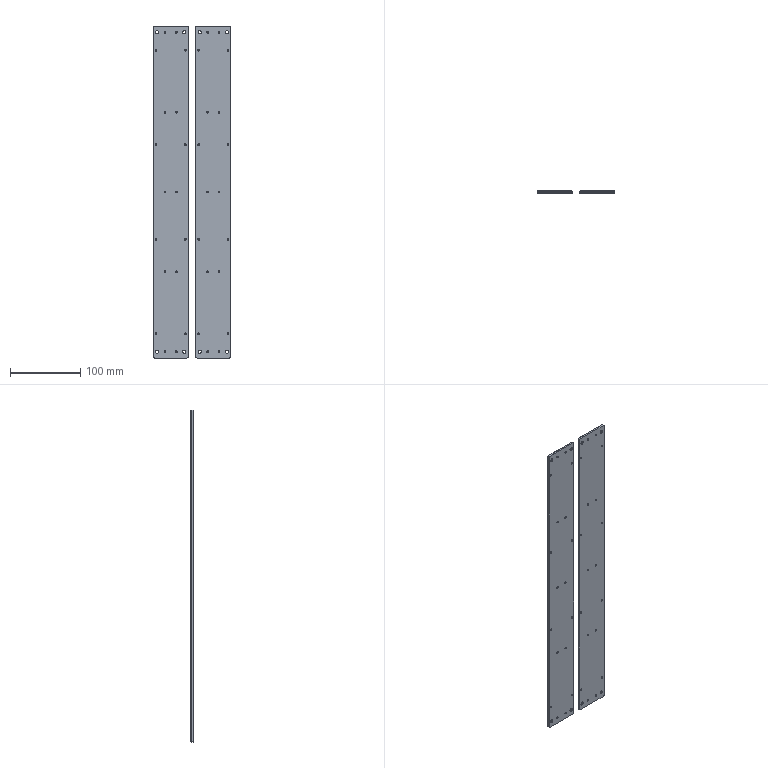Part | 2 solids | 88 faces | box 111 x 3 x 474 mm | volume 140633 mm3 | cylinder 52 | plane 20 | cone 16 | commonest cylinder face diameters 2.5 x36 4 x8 4.5 x8